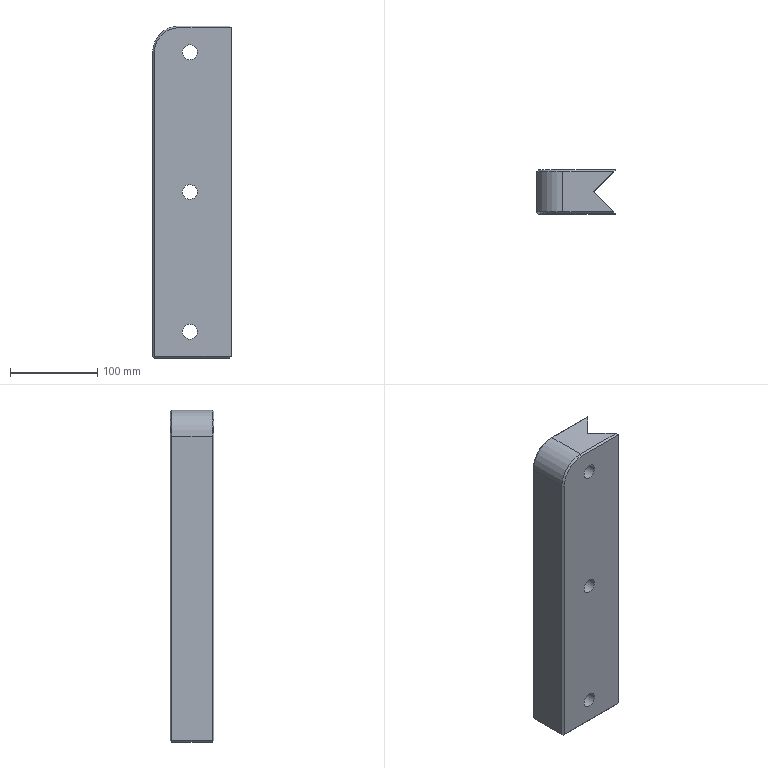Part | Creo | features DATUM PLANE 3, CURVE 2, CHAMFER 1, COORDINATE SYSTEM 1, CUT 1, PROTRUSION 1, ROUND 1 | 1 solid | 23 faces | box 90 x 50 x 380 mm | volume 1426529 mm3 | plane 14 | cylinder 7 | cone 2 | commonest cylinder face diameters 17 x6 60 x1
STEP:
#1=CARTESIAN_POINT('',(0.,0.,0.));
#2=DIRECTION('',(0.,0.,1.));
#3=DIRECTION('',(1.,0.,0.));
#4=AXIS2_PLACEMENT_3D('',#1,#2,#3);
#5=CARTESIAN_POINT('',(-40.5,23.,0.));
#6=VERTEX_POINT('',#5);
#7=CARTESIAN_POINT('',(45.5,23.,0.));
#8=VERTEX_POINT('',#7);
#9=CARTESIAN_POINT('',(-40.5,23.,0.));
#10=DIRECTION('',(1.,0.,0.));
#11=VECTOR('',#10,86.);
#12=LINE('',#9,#11);
#13=EDGE_CURVE('',#6,#8,#12,.T.);
#14=ORIENTED_EDGE('',*,*,#13,.F.);
#15=CARTESIAN_POINT('',(-40.5,-23.,0.));
#16=VERTEX_POINT('',#15);
#17=CARTESIAN_POINT('',(-40.5,-23.,0.));
#18=DIRECTION('',(0.,1.,0.));
#19=VECTOR('',#18,46.);
#20=LINE('',#17,#19);
#21=EDGE_CURVE('',#16,#6,#20,.T.);
#22=ORIENTED_EDGE('',*,*,#21,.F.);
#23=CARTESIAN_POINT('',(45.5,-23.,0.));
#24=VERTEX_POINT('',#23);
#25=CARTESIAN_POINT('',(45.5,-23.,0.));
#26=DIRECTION('',(-1.,0.,0.));
#27=VECTOR('',#26,86.);
#28=LINE('',#25,#27);
#29=EDGE_CURVE('',#24,#16,#28,.T.);
#30=ORIENTED_EDGE('',*,*,#29,.F.);
#31=CARTESIAN_POINT('',(22.5,0.,0.));
#32=VERTEX_POINT('',#31);
#33=CARTESIAN_POINT('',(45.5,-23.,0.));
#34=DIRECTION('',(-0.7071,0.7071,0.));
#35=VECTOR('',#34,32.527);
#36=LINE('',#33,#35);
#37=EDGE_CURVE('',#24,#32,#36,.T.);
#38=ORIENTED_EDGE('',*,*,#37,.T.);
#39=CARTESIAN_POINT('',(22.5,0.,0.));
#40=DIRECTION('',(0.7071,0.7071,0.));
#41=VECTOR('',#40,32.527);
#42=LINE('',#39,#41);
#43=EDGE_CURVE('',#32,#8,#42,.T.);
#44=ORIENTED_EDGE('',*,*,#43,.T.);
#45=EDGE_LOOP('',(#14,#22,#30,#38,#44));
#46=FACE_OUTER_BOUND('',#45,.F.);
#47=CARTESIAN_POINT('',(0.,0.,0.));
#48=DIRECTION('',(0.,0.,1.));
#49=DIRECTION('',(1.,0.,0.));
#50=AXIS2_PLACEMENT_3D('',#47,#48,#49);
#51=PLANE('',#50);
#52=ADVANCED_FACE('',(#46),#51,.F.);
#53=CARTESIAN_POINT('',(47.5,25.,2.));
#54=VERTEX_POINT('',#53);
#55=CARTESIAN_POINT('',(45.5,23.,0.));
#56=DIRECTION('',(0.5774,0.5774,0.5774));
#57=VECTOR('',#56,3.464);
#58=LINE('',#55,#57);
#59=EDGE_CURVE('',#8,#54,#58,.T.);
#60=ORIENTED_EDGE('',*,*,#59,.T.);
#61=CARTESIAN_POINT('',(-40.5,25.,2.));
#62=VERTEX_POINT('',#61);
#63=CARTESIAN_POINT('',(-40.5,25.,2.));
#64=DIRECTION('',(1.,0.,0.));
#65=VECTOR('',#64,88.);
#66=LINE('',#63,#65);
#67=EDGE_CURVE('',#62,#54,#66,.T.);
#68=ORIENTED_EDGE('',*,*,#67,.F.);
#69=CARTESIAN_POINT('',(-41.5,24.,1.));
#70=VERTEX_POINT('',#69);
#71=CARTESIAN_POINT('',(-40.5,25.,2.));
#72=DIRECTION('',(-0.5774,-0.5774,-0.5774));
#73=VECTOR('',#72,1.732);
#74=LINE('',#71,#73);
#75=EDGE_CURVE('',#62,#70,#74,.T.);
#76=ORIENTED_EDGE('',*,*,#75,.T.);
#77=CARTESIAN_POINT('',(-40.5,23.,0.));
#78=DIRECTION('',(-0.5774,0.5774,0.5774));
#79=VECTOR('',#78,1.732);
#80=LINE('',#77,#79);
#81=EDGE_CURVE('',#6,#70,#80,.T.);
#82=ORIENTED_EDGE('',*,*,#81,.F.);
#83=ORIENTED_EDGE('',*,*,#13,.T.);
#84=EDGE_LOOP('',(#60,#68,#76,#82,#83));
#85=FACE_OUTER_BOUND('',#84,.F.);
#86=CARTESIAN_POINT('',(1.5,24.,1.));
#87=DIRECTION('',(0.,0.7071,-0.7071));
#88=DIRECTION('',(0.,0.7071,0.7071));
#89=AXIS2_PLACEMENT_3D('',#86,#87,#88);
#90=PLANE('',#89);
#91=ADVANCED_FACE('',(#85),#90,.T.);
#92=ORIENTED_EDGE('',*,*,#59,.F.);
#93=ORIENTED_EDGE('',*,*,#43,.F.);
#94=CARTESIAN_POINT('',(22.5,0.,380.));
#95=VERTEX_POINT('',#94);
#96=CARTESIAN_POINT('',(22.5,0.,0.));
#97=DIRECTION('',(0.,0.,1.));
#98=VECTOR('',#97,380.);
#99=LINE('',#96,#98);
#100=EDGE_CURVE('',#32,#95,#99,.T.);
#101=ORIENTED_EDGE('',*,*,#100,.T.);
#102=CARTESIAN_POINT('',(45.5,23.,380.));
#103=VERTEX_POINT('',#102);
#104=CARTESIAN_POINT('',(22.5,0.,380.));
#105=DIRECTION('',(0.7071,0.7071,0.));
#106=VECTOR('',#105,32.527);
#107=LINE('',#104,#106);
#108=EDGE_CURVE('',#95,#103,#107,.T.);
#109=ORIENTED_EDGE('',*,*,#108,.T.);
#110=CARTESIAN_POINT('',(47.5,25.,378.));
#111=VERTEX_POINT('',#110);
#112=CARTESIAN_POINT('',(47.5,25.,378.));
#113=DIRECTION('',(-0.5774,-0.5774,0.5774));
#114=VECTOR('',#113,3.464);
#115=LINE('',#112,#114);
#116=EDGE_CURVE('',#111,#103,#115,.T.);
#117=ORIENTED_EDGE('',*,*,#116,.F.);
#118=CARTESIAN_POINT('',(47.5,25.,2.));
#119=DIRECTION('',(0.,0.,1.));
#120=VECTOR('',#119,376.);
#121=LINE('',#118,#120);
#122=EDGE_CURVE('',#54,#111,#121,.T.);
#123=ORIENTED_EDGE('',*,*,#122,.F.);
#124=EDGE_LOOP('',(#92,#93,#101,#109,#117,#123));
#125=FACE_OUTER_BOUND('',#124,.F.);
#126=CARTESIAN_POINT('',(22.5,0.,0.));
#127=DIRECTION('',(0.7071,-0.7071,0.));
#128=DIRECTION('',(0.7071,0.7071,0.));
#129=AXIS2_PLACEMENT_3D('',#126,#127,#128);
#130=PLANE('',#129);
#131=ADVANCED_FACE('',(#125),#130,.T.);
#132=CARTESIAN_POINT('',(47.5,-25.,2.));
#133=VERTEX_POINT('',#132);
#134=CARTESIAN_POINT('',(47.5,-25.,2.));
#135=DIRECTION('',(-0.5774,0.5774,-0.5774));
#136=VECTOR('',#135,3.464);
#137=LINE('',#134,#136);
#138=EDGE_CURVE('',#133,#24,#137,.T.);
#139=ORIENTED_EDGE('',*,*,#138,.F.);
#140=CARTESIAN_POINT('',(47.5,-25.,378.));
#141=VERTEX_POINT('',#140);
#142=CARTESIAN_POINT('',(47.5,-25.,2.));
#143=DIRECTION('',(0.,0.,1.));
#144=VECTOR('',#143,376.);
#145=LINE('',#142,#144);
#146=EDGE_CURVE('',#133,#141,#145,.T.);
#147=ORIENTED_EDGE('',*,*,#146,.T.);
#148=CARTESIAN_POINT('',(45.5,-23.,380.));
#149=VERTEX_POINT('',#148);
#150=CARTESIAN_POINT('',(45.5,-23.,380.));
#151=DIRECTION('',(0.5774,-0.5774,-0.5774));
#152=VECTOR('',#151,3.464);
#153=LINE('',#150,#152);
#154=EDGE_CURVE('',#149,#141,#153,.T.);
#155=ORIENTED_EDGE('',*,*,#154,.F.);
#156=CARTESIAN_POINT('',(45.5,-23.,380.));
#157=DIRECTION('',(-0.7071,0.7071,0.));
#158=VECTOR('',#157,32.527);
#159=LINE('',#156,#158);
#160=EDGE_CURVE('',#149,#95,#159,.T.);
#161=ORIENTED_EDGE('',*,*,#160,.T.);
#162=ORIENTED_EDGE('',*,*,#100,.F.);
#163=ORIENTED_EDGE('',*,*,#37,.F.);
#164=EDGE_LOOP('',(#139,#147,#155,#161,#162,#163));
#165=FACE_OUTER_BOUND('',#164,.F.);
#166=CARTESIAN_POINT('',(47.5,-25.,0.));
#167=DIRECTION('',(0.7071,0.7071,0.));
#168=DIRECTION('',(-0.7071,0.7071,0.));
#169=AXIS2_PLACEMENT_3D('',#166,#167,#168);
#170=PLANE('',#169);
#171=ADVANCED_FACE('',(#165),#170,.T.);
#172=ORIENTED_EDGE('',*,*,#138,.T.);
#173=ORIENTED_EDGE('',*,*,#29,.T.);
#174=CARTESIAN_POINT('',(-41.5,-24.,1.));
#175=VERTEX_POINT('',#174);
#176=CARTESIAN_POINT('',(-41.5,-24.,1.));
#177=DIRECTION('',(0.5774,0.5774,-0.5774));
#178=VECTOR('',#177,1.732);
#179=LINE('',#176,#178);
#180=EDGE_CURVE('',#175,#16,#179,.T.);
#181=ORIENTED_EDGE('',*,*,#180,.F.);
#182=CARTESIAN_POINT('',(-40.5,-25.,2.));
#183=VERTEX_POINT('',#182);
#184=CARTESIAN_POINT('',(-40.5,-25.,2.));
#185=DIRECTION('',(-0.5774,0.5774,-0.5774));
#186=VECTOR('',#185,1.732);
#187=LINE('',#184,#186);
#188=EDGE_CURVE('',#183,#175,#187,.T.);
#189=ORIENTED_EDGE('',*,*,#188,.F.);
#190=CARTESIAN_POINT('',(47.5,-25.,2.));
#191=DIRECTION('',(-1.,0.,0.));
#192=VECTOR('',#191,88.);
#193=LINE('',#190,#192);
#194=EDGE_CURVE('',#133,#183,#193,.T.);
#195=ORIENTED_EDGE('',*,*,#194,.F.);
#196=EDGE_LOOP('',(#172,#173,#181,#189,#195));
#197=FACE_OUTER_BOUND('',#196,.F.);
#198=CARTESIAN_POINT('',(1.5,-24.,1.));
#199=DIRECTION('',(0.,-0.7071,-0.7071));
#200=DIRECTION('',(0.,-0.7071,0.7071));
#201=AXIS2_PLACEMENT_3D('',#198,#199,#200);
#202=PLANE('',#201);
#203=ADVANCED_FACE('',(#197),#202,.T.);
#204=CARTESIAN_POINT('',(-42.5,-23.,2.));
#205=VERTEX_POINT('',#204);
#206=CARTESIAN_POINT('',(-42.5,23.,2.));
#207=VERTEX_POINT('',#206);
#208=CARTESIAN_POINT('',(-42.5,-23.,2.));
#209=DIRECTION('',(0.,1.,0.));
#210=VECTOR('',#209,46.);
#211=LINE('',#208,#210);
#212=EDGE_CURVE('',#205,#207,#211,.T.);
#213=ORIENTED_EDGE('',*,*,#212,.F.);
#214=CARTESIAN_POINT('',(-42.5,-23.,2.));
#215=DIRECTION('',(0.5774,-0.5774,-0.5774));
#216=VECTOR('',#215,1.732);
#217=LINE('',#214,#216);
#218=EDGE_CURVE('',#205,#175,#217,.T.);
#219=ORIENTED_EDGE('',*,*,#218,.T.);
#220=ORIENTED_EDGE('',*,*,#180,.T.);
#221=ORIENTED_EDGE('',*,*,#21,.T.);
#222=ORIENTED_EDGE('',*,*,#81,.T.);
#223=CARTESIAN_POINT('',(-41.5,24.,1.));
#224=DIRECTION('',(-0.5774,-0.5774,0.5774));
#225=VECTOR('',#224,1.732);
#226=LINE('',#223,#225);
#227=EDGE_CURVE('',#70,#207,#226,.T.);
#228=ORIENTED_EDGE('',*,*,#227,.T.);
#229=EDGE_LOOP('',(#213,#219,#220,#221,#222,#228));
#230=FACE_OUTER_BOUND('',#229,.F.);
#231=CARTESIAN_POINT('',(-41.5,0.,1.));
#232=DIRECTION('',(-0.7071,0.,-0.7071));
#233=DIRECTION('',(-0.7071,0.,0.7071));
#234=AXIS2_PLACEMENT_3D('',#231,#232,#233);
#235=PLANE('',#234);
#236=ADVANCED_FACE('',(#230),#235,.T.);
#237=CARTESIAN_POINT('',(-42.5,23.,350.));
#238=VERTEX_POINT('',#237);
#239=CARTESIAN_POINT('',(-42.5,23.,350.));
#240=DIRECTION('',(0.,0.,-1.));
#241=VECTOR('',#240,348.);
#242=LINE('',#239,#241);
#243=EDGE_CURVE('',#238,#207,#242,.T.);
#244=ORIENTED_EDGE('',*,*,#243,.F.);
#245=CARTESIAN_POINT('',(-42.5,-23.,350.));
#246=VERTEX_POINT('',#245);
#247=CARTESIAN_POINT('',(-42.5,23.,350.));
#248=DIRECTION('',(0.,-1.,0.));
#249=VECTOR('',#248,46.);
#250=LINE('',#247,#249);
#251=EDGE_CURVE('',#238,#246,#250,.T.);
#252=ORIENTED_EDGE('',*,*,#251,.T.);
#253=CARTESIAN_POINT('',(-42.5,-23.,350.));
#254=DIRECTION('',(0.,0.,-1.));
#255=VECTOR('',#254,348.);
#256=LINE('',#253,#255);
#257=EDGE_CURVE('',#246,#205,#256,.T.);
#258=ORIENTED_EDGE('',*,*,#257,.T.);
#259=ORIENTED_EDGE('',*,*,#212,.T.);
#260=EDGE_LOOP('',(#244,#252,#258,#259));
#261=FACE_OUTER_BOUND('',#260,.F.);
#262=CARTESIAN_POINT('',(-42.5,25.,0.));
#263=DIRECTION('',(-1.,0.,0.));
#264=DIRECTION('',(0.,-1.,0.));
#265=AXIS2_PLACEMENT_3D('',#262,#263,#264);
#266=PLANE('',#265);
#267=ADVANCED_FACE('',(#261),#266,.T.);
#268=CARTESIAN_POINT('',(-40.5,25.,350.));
#269=VERTEX_POINT('',#268);
#270=CARTESIAN_POINT('',(-40.5,25.,350.));
#271=DIRECTION('',(0.,0.,-1.));
#272=VECTOR('',#271,348.);
#273=LINE('',#270,#272);
#274=EDGE_CURVE('',#269,#62,#273,.T.);
#275=ORIENTED_EDGE('',*,*,#274,.F.);
#276=CARTESIAN_POINT('',(-42.5,23.,350.));
#277=DIRECTION('',(0.7071,0.7071,-0.00000001));
#278=VECTOR('',#277,2.828);
#279=LINE('',#276,#278);
#280=EDGE_CURVE('',#238,#269,#279,.T.);
#281=ORIENTED_EDGE('',*,*,#280,.F.);
#282=ORIENTED_EDGE('',*,*,#243,.T.);
#283=ORIENTED_EDGE('',*,*,#227,.F.);
#284=ORIENTED_EDGE('',*,*,#75,.F.);
#285=EDGE_LOOP('',(#275,#281,#282,#283,#284));
#286=FACE_OUTER_BOUND('',#285,.F.);
#287=CARTESIAN_POINT('',(-41.5,24.,175.));
#288=DIRECTION('',(-0.7071,0.7071,0.));
#289=DIRECTION('',(0.7071,0.7071,0.));
#290=AXIS2_PLACEMENT_3D('',#287,#288,#289);
#291=PLANE('',#290);
#292=ADVANCED_FACE('',(#286),#291,.T.);
#293=ORIENTED_EDGE('',*,*,#67,.T.);
#294=ORIENTED_EDGE('',*,*,#122,.T.);
#295=CARTESIAN_POINT('',(-12.5,25.,378.));
#296=VERTEX_POINT('',#295);
#297=CARTESIAN_POINT('',(47.5,25.,378.));
#298=DIRECTION('',(-1.,0.,0.));
#299=VECTOR('',#298,60.);
#300=LINE('',#297,#299);
#301=EDGE_CURVE('',#111,#296,#300,.T.);
#302=ORIENTED_EDGE('',*,*,#301,.T.);
#303=CARTESIAN_POINT('',(-12.5,25.,350.));
#304=DIRECTION('',(0.,-1.,0.));
#305=DIRECTION('',(0.,0.,1.));
#306=AXIS2_PLACEMENT_3D('',#303,#304,#305);
#307=CIRCLE('',#306,28.);
#308=EDGE_CURVE('',#296,#269,#307,.T.);
#309=ORIENTED_EDGE('',*,*,#308,.T.);
#310=ORIENTED_EDGE('',*,*,#274,.T.);
#311=EDGE_LOOP('',(#293,#294,#302,#309,#310));
#312=FACE_OUTER_BOUND('',#311,.F.);
#313=CARTESIAN_POINT('',(8.5,25.,190.));
#314=VERTEX_POINT('',#313);
#315=CARTESIAN_POINT('',(-8.5,25.,190.));
#316=VERTEX_POINT('',#315);
#317=CARTESIAN_POINT('',(0.,25.,190.));
#318=DIRECTION('',(0.,-1.,0.));
#319=DIRECTION('',(1.,0.,0.));
#320=AXIS2_PLACEMENT_3D('',#317,#318,#319);
#321=CIRCLE('',#320,8.5);
#322=EDGE_CURVE('',#314,#316,#321,.T.);
#323=ORIENTED_EDGE('',*,*,#322,.F.);
#324=CARTESIAN_POINT('',(0.,25.,190.));
#325=DIRECTION('',(0.,-1.,0.));
#326=DIRECTION('',(-1.,0.,0.));
#327=AXIS2_PLACEMENT_3D('',#324,#325,#326);
#328=CIRCLE('',#327,8.5);
#329=EDGE_CURVE('',#316,#314,#328,.T.);
#330=ORIENTED_EDGE('',*,*,#329,.F.);
#331=EDGE_LOOP('',(#323,#330));
#332=FACE_BOUND('',#331,.F.);
#333=CARTESIAN_POINT('',(8.5,25.,30.));
#334=VERTEX_POINT('',#333);
#335=CARTESIAN_POINT('',(-8.5,25.,30.));
#336=VERTEX_POINT('',#335);
#337=CARTESIAN_POINT('',(0.,25.,30.));
#338=DIRECTION('',(0.,-1.,0.));
#339=DIRECTION('',(1.,0.,0.));
#340=AXIS2_PLACEMENT_3D('',#337,#338,#339);
#341=CIRCLE('',#340,8.5);
#342=EDGE_CURVE('',#334,#336,#341,.T.);
#343=ORIENTED_EDGE('',*,*,#342,.F.);
#344=CARTESIAN_POINT('',(0.,25.,30.));
#345=DIRECTION('',(0.,-1.,0.));
#346=DIRECTION('',(-1.,0.,0.));
#347=AXIS2_PLACEMENT_3D('',#344,#345,#346);
#348=CIRCLE('',#347,8.5);
#349=EDGE_CURVE('',#336,#334,#348,.T.);
#350=ORIENTED_EDGE('',*,*,#349,.F.);
#351=EDGE_LOOP('',(#343,#350));
#352=FACE_BOUND('',#351,.F.);
#353=CARTESIAN_POINT('',(8.5,25.,350.));
#354=VERTEX_POINT('',#353);
#355=CARTESIAN_POINT('',(-8.5,25.,350.));
#356=VERTEX_POINT('',#355);
#357=CARTESIAN_POINT('',(0.,25.,350.));
#358=DIRECTION('',(0.,-1.,0.));
#359=DIRECTION('',(1.,0.,0.));
#360=AXIS2_PLACEMENT_3D('',#357,#358,#359);
#361=CIRCLE('',#360,8.5);
#362=EDGE_CURVE('',#354,#356,#361,.T.);
#363=ORIENTED_EDGE('',*,*,#362,.F.);
#364=CARTESIAN_POINT('',(0.,25.,350.));
#365=DIRECTION('',(0.,-1.,0.));
#366=DIRECTION('',(-1.,0.,0.));
#367=AXIS2_PLACEMENT_3D('',#364,#365,#366);
#368=CIRCLE('',#367,8.5);
#369=EDGE_CURVE('',#356,#354,#368,.T.);
#370=ORIENTED_EDGE('',*,*,#369,.F.);
#371=EDGE_LOOP('',(#363,#370));
#372=FACE_BOUND('',#371,.F.);
#373=CARTESIAN_POINT('',(47.5,25.,0.));
#374=DIRECTION('',(0.,1.,0.));
#375=DIRECTION('',(-1.,0.,0.));
#376=AXIS2_PLACEMENT_3D('',#373,#374,#375);
#377=PLANE('',#376);
#378=ADVANCED_FACE('',(#312,#332,#352,#372),#377,.T.);
#379=CARTESIAN_POINT('',(8.5,-25.,350.));
#380=VERTEX_POINT('',#379);
#381=CARTESIAN_POINT('',(-8.5,-25.,350.));
#382=VERTEX_POINT('',#381);
#383=CARTESIAN_POINT('',(0.,-25.,350.));
#384=DIRECTION('',(0.,-1.,0.));
#385=DIRECTION('',(1.,0.,0.));
#386=AXIS2_PLACEMENT_3D('',#383,#384,#385);
#387=CIRCLE('',#386,8.5);
#388=EDGE_CURVE('',#380,#382,#387,.T.);
#389=ORIENTED_EDGE('',*,*,#388,.F.);
#390=CARTESIAN_POINT('',(8.5,-25.,350.));
#391=DIRECTION('',(0.,1.,0.));
#392=VECTOR('',#391,50.);
#393=LINE('',#390,#392);
#394=EDGE_CURVE('',#380,#354,#393,.T.);
#395=ORIENTED_EDGE('',*,*,#394,.T.);
#396=ORIENTED_EDGE('',*,*,#362,.T.);
#397=CARTESIAN_POINT('',(-8.5,-25.,350.));
#398=DIRECTION('',(0.,1.,0.));
#399=VECTOR('',#398,50.);
#400=LINE('',#397,#399);
#401=EDGE_CURVE('',#382,#356,#400,.T.);
#402=ORIENTED_EDGE('',*,*,#401,.F.);
#403=EDGE_LOOP('',(#389,#395,#396,#402));
#404=FACE_OUTER_BOUND('',#403,.F.);
#405=CARTESIAN_POINT('',(0.,-25.,350.));
#406=DIRECTION('',(0.,-1.,0.));
#407=DIRECTION('',(1.,0.,0.));
#408=AXIS2_PLACEMENT_3D('',#405,#406,#407);
#409=CYLINDRICAL_SURFACE('',#408,8.5);
#410=ADVANCED_FACE('',(#404),#409,.F.);
#411=ORIENTED_EDGE('',*,*,#194,.T.);
#412=CARTESIAN_POINT('',(-40.5,-25.,350.));
#413=VERTEX_POINT('',#412);
#414=CARTESIAN_POINT('',(-40.5,-25.,350.));
#415=DIRECTION('',(0.,0.,-1.));
#416=VECTOR('',#415,348.);
#417=LINE('',#414,#416);
#418=EDGE_CURVE('',#413,#183,#417,.T.);
#419=ORIENTED_EDGE('',*,*,#418,.F.);
#420=CARTESIAN_POINT('',(-12.5,-25.,378.));
#421=VERTEX_POINT('',#420);
#422=CARTESIAN_POINT('',(-12.5,-25.,350.));
#423=DIRECTION('',(0.,-1.,0.));
#424=DIRECTION('',(0.,0.,1.));
#425=AXIS2_PLACEMENT_3D('',#422,#423,#424);
#426=CIRCLE('',#425,28.);
#427=EDGE_CURVE('',#421,#413,#426,.T.);
#428=ORIENTED_EDGE('',*,*,#427,.F.);
#429=CARTESIAN_POINT('',(47.5,-25.,378.));
#430=DIRECTION('',(-1.,0.,0.));
#431=VECTOR('',#430,60.);
#432=LINE('',#429,#431);
#433=EDGE_CURVE('',#141,#421,#432,.T.);
#434=ORIENTED_EDGE('',*,*,#433,.F.);
#435=ORIENTED_EDGE('',*,*,#146,.F.);
#436=EDGE_LOOP('',(#411,#419,#428,#434,#435));
#437=FACE_OUTER_BOUND('',#436,.F.);
#438=CARTESIAN_POINT('',(8.5,-25.,190.));
#439=VERTEX_POINT('',#438);
#440=CARTESIAN_POINT('',(-8.5,-25.,190.));
#441=VERTEX_POINT('',#440);
#442=CARTESIAN_POINT('',(0.,-25.,190.));
#443=DIRECTION('',(0.,-1.,0.));
#444=DIRECTION('',(1.,0.,0.));
#445=AXIS2_PLACEMENT_3D('',#442,#443,#444);
#446=CIRCLE('',#445,8.5);
#447=EDGE_CURVE('',#439,#441,#446,.T.);
#448=ORIENTED_EDGE('',*,*,#447,.T.);
#449=CARTESIAN_POINT('',(0.,-25.,190.));
#450=DIRECTION('',(0.,-1.,0.));
#451=DIRECTION('',(-1.,0.,0.));
#452=AXIS2_PLACEMENT_3D('',#449,#450,#451);
#453=CIRCLE('',#452,8.5);
#454=EDGE_CURVE('',#441,#439,#453,.T.);
#455=ORIENTED_EDGE('',*,*,#454,.T.);
#456=EDGE_LOOP('',(#448,#455));
#457=FACE_BOUND('',#456,.F.);
#458=CARTESIAN_POINT('',(8.5,-25.,30.));
#459=VERTEX_POINT('',#458);
#460=CARTESIAN_POINT('',(-8.5,-25.,30.));
#461=VERTEX_POINT('',#460);
#462=CARTESIAN_POINT('',(0.,-25.,30.));
#463=DIRECTION('',(0.,-1.,0.));
#464=DIRECTION('',(1.,0.,0.));
#465=AXIS2_PLACEMENT_3D('',#462,#463,#464);
#466=CIRCLE('',#465,8.5);
#467=EDGE_CURVE('',#459,#461,#466,.T.);
#468=ORIENTED_EDGE('',*,*,#467,.T.);
#469=CARTESIAN_POINT('',(0.,-25.,30.));
#470=DIRECTION('',(0.,-1.,0.));
#471=DIRECTION('',(-1.,0.,0.));
#472=AXIS2_PLACEMENT_3D('',#469,#470,#471);
#473=CIRCLE('',#472,8.5);
#474=EDGE_CURVE('',#461,#459,#473,.T.);
#475=ORIENTED_EDGE('',*,*,#474,.T.);
#476=EDGE_LOOP('',(#468,#475));
#477=FACE_BOUND('',#476,.F.);
#478=ORIENTED_EDGE('',*,*,#388,.T.);
#479=CARTESIAN_POINT('',(0.,-25.,350.));
#480=DIRECTION('',(0.,-1.,0.));
#481=DIRECTION('',(-1.,0.,0.));
#482=AXIS2_PLACEMENT_3D('',#479,#480,#481);
#483=CIRCLE('',#482,8.5);
#484=EDGE_CURVE('',#382,#380,#483,.T.);
#485=ORIENTED_EDGE('',*,*,#484,.T.);
#486=EDGE_LOOP('',(#478,#485));
#487=FACE_BOUND('',#486,.F.);
#488=CARTESIAN_POINT('',(-42.5,-25.,0.));
#489=DIRECTION('',(0.,-1.,0.));
#490=DIRECTION('',(1.,0.,0.));
#491=AXIS2_PLACEMENT_3D('',#488,#489,#490);
#492=PLANE('',#491);
#493=ADVANCED_FACE('',(#437,#457,#477,#487),#492,.T.);
#494=ORIENTED_EDGE('',*,*,#484,.F.);
#495=ORIENTED_EDGE('',*,*,#401,.T.);
#496=ORIENTED_EDGE('',*,*,#369,.T.);
#497=ORIENTED_EDGE('',*,*,#394,.F.);
#498=EDGE_LOOP('',(#494,#495,#496,#497));
#499=FACE_OUTER_BOUND('',#498,.F.);
#500=CARTESIAN_POINT('',(0.,-25.,350.));
#501=DIRECTION('',(0.,-1.,0.));
#502=DIRECTION('',(1.,0.,0.));
#503=AXIS2_PLACEMENT_3D('',#500,#501,#502);
#504=CYLINDRICAL_SURFACE('',#503,8.5);
#505=ADVANCED_FACE('',(#499),#504,.F.);
#506=ORIENTED_EDGE('',*,*,#447,.F.);
#507=CARTESIAN_POINT('',(8.5,-25.,190.));
#508=DIRECTION('',(0.,1.,0.));
#509=VECTOR('',#508,50.);
#510=LINE('',#507,#509);
#511=EDGE_CURVE('',#439,#314,#510,.T.);
#512=ORIENTED_EDGE('',*,*,#511,.T.);
#513=ORIENTED_EDGE('',*,*,#322,.T.);
#514=CARTESIAN_POINT('',(-8.5,-25.,190.));
#515=DIRECTION('',(0.,1.,0.));
#516=VECTOR('',#515,50.);
#517=LINE('',#514,#516);
#518=EDGE_CURVE('',#441,#316,#517,.T.);
#519=ORIENTED_EDGE('',*,*,#518,.F.);
#520=EDGE_LOOP('',(#506,#512,#513,#519));
#521=FACE_OUTER_BOUND('',#520,.F.);
#522=CARTESIAN_POINT('',(0.,-25.,190.));
#523=DIRECTION('',(0.,-1.,0.));
#524=DIRECTION('',(1.,0.,0.));
#525=AXIS2_PLACEMENT_3D('',#522,#523,#524);
#526=CYLINDRICAL_SURFACE('',#525,8.5);
#527=ADVANCED_FACE('',(#521),#526,.F.);
#528=ORIENTED_EDGE('',*,*,#454,.F.);
#529=ORIENTED_EDGE('',*,*,#518,.T.);
#530=ORIENTED_EDGE('',*,*,#329,.T.);
#531=ORIENTED_EDGE('',*,*,#511,.F.);
#532=EDGE_LOOP('',(#528,#529,#530,#531));
#533=FACE_OUTER_BOUND('',#532,.F.);
#534=CARTESIAN_POINT('',(0.,-25.,190.));
#535=DIRECTION('',(0.,-1.,0.));
#536=DIRECTION('',(1.,0.,0.));
#537=AXIS2_PLACEMENT_3D('',#534,#535,#536);
#538=CYLINDRICAL_SURFACE('',#537,8.5);
#539=ADVANCED_FACE('',(#533),#538,.F.);
#540=ORIENTED_EDGE('',*,*,#467,.F.);
#541=CARTESIAN_POINT('',(8.5,-25.,30.));
#542=DIRECTION('',(0.,1.,0.));
#543=VECTOR('',#542,50.);
#544=LINE('',#541,#543);
#545=EDGE_CURVE('',#459,#334,#544,.T.);
#546=ORIENTED_EDGE('',*,*,#545,.T.);
#547=ORIENTED_EDGE('',*,*,#342,.T.);
#548=CARTESIAN_POINT('',(-8.5,-25.,30.));
#549=DIRECTION('',(0.,1.,0.));
#550=VECTOR('',#549,50.);
#551=LINE('',#548,#550);
#552=EDGE_CURVE('',#461,#336,#551,.T.);
#553=ORIENTED_EDGE('',*,*,#552,.F.);
#554=EDGE_LOOP('',(#540,#546,#547,#553));
#555=FACE_OUTER_BOUND('',#554,.F.);
#556=CARTESIAN_POINT('',(0.,-25.,30.));
#557=DIRECTION('',(0.,-1.,0.));
#558=DIRECTION('',(1.,0.,0.));
#559=AXIS2_PLACEMENT_3D('',#556,#557,#558);
#560=CYLINDRICAL_SURFACE('',#559,8.5);
#561=ADVANCED_FACE('',(#555),#560,.F.);
#562=ORIENTED_EDGE('',*,*,#474,.F.);
#563=ORIENTED_EDGE('',*,*,#552,.T.);
#564=ORIENTED_EDGE('',*,*,#349,.T.);
#565=ORIENTED_EDGE('',*,*,#545,.F.);
#566=EDGE_LOOP('',(#562,#563,#564,#565));
#567=FACE_OUTER_BOUND('',#566,.F.);
#568=CARTESIAN_POINT('',(0.,-25.,30.));
#569=DIRECTION('',(0.,-1.,0.));
#570=DIRECTION('',(1.,0.,0.));
#571=AXIS2_PLACEMENT_3D('',#568,#569,#570);
#572=CYLINDRICAL_SURFACE('',#571,8.5);
#573=ADVANCED_FACE('',(#567),#572,.F.);
#574=ORIENTED_EDGE('',*,*,#257,.F.);
#575=CARTESIAN_POINT('',(-40.5,-25.,350.));
#576=DIRECTION('',(-0.7071,0.7071,0.00000001));
#577=VECTOR('',#576,2.828);
#578=LINE('',#575,#577);
#579=EDGE_CURVE('',#413,#246,#578,.T.);
#580=ORIENTED_EDGE('',*,*,#579,.F.);
#581=ORIENTED_EDGE('',*,*,#418,.T.);
#582=ORIENTED_EDGE('',*,*,#188,.T.);
#583=ORIENTED_EDGE('',*,*,#218,.F.);
#584=EDGE_LOOP('',(#574,#580,#581,#582,#583));
#585=FACE_OUTER_BOUND('',#584,.F.);
#586=CARTESIAN_POINT('',(-41.5,-24.,175.));
#587=DIRECTION('',(-0.7071,-0.7071,0.));
#588=DIRECTION('',(-0.7071,0.7071,0.));
#589=AXIS2_PLACEMENT_3D('',#586,#587,#588);
#590=PLANE('',#589);
#591=ADVANCED_FACE('',(#585),#590,.T.);
#592=ORIENTED_EDGE('',*,*,#427,.T.);
#593=ORIENTED_EDGE('',*,*,#579,.T.);
#594=CARTESIAN_POINT('',(-12.5,-23.,380.));
#595=VERTEX_POINT('',#594);
#596=CARTESIAN_POINT('',(-12.5,-23.,350.));
#597=DIRECTION('',(0.,-1.,0.));
#598=DIRECTION('',(0.,0.,1.));
#599=AXIS2_PLACEMENT_3D('',#596,#597,#598);
#600=CIRCLE('',#599,30.);
#601=EDGE_CURVE('',#595,#246,#600,.T.);
#602=ORIENTED_EDGE('',*,*,#601,.F.);
#603=CARTESIAN_POINT('',(-12.5,-25.,378.));
#604=DIRECTION('',(0.000000032,0.7071,0.7071));
#605=VECTOR('',#604,2.828);
#606=LINE('',#603,#605);
#607=EDGE_CURVE('',#421,#595,#606,.T.);
#608=ORIENTED_EDGE('',*,*,#607,.F.);
#609=EDGE_LOOP('',(#592,#593,#602,#608));
#610=FACE_OUTER_BOUND('',#609,.F.);
#611=CARTESIAN_POINT('',(-12.5,-24.,350.));
#612=DIRECTION('',(0.,1.,0.));
#613=DIRECTION('',(0.,0.,-1.));
#614=AXIS2_PLACEMENT_3D('',#611,#612,#613);
#615=CONICAL_SURFACE('',#614,29.,45.);
#616=ADVANCED_FACE('',(#610),#615,.T.);
#617=CARTESIAN_POINT('',(-12.5,23.,380.));
#618=VERTEX_POINT('',#617);
#619=CARTESIAN_POINT('',(-12.5,23.,350.));
#620=DIRECTION('',(0.,-1.,0.));
#621=DIRECTION('',(0.,0.,1.));
#622=AXIS2_PLACEMENT_3D('',#619,#620,#621);
#623=CIRCLE('',#622,30.);
#624=EDGE_CURVE('',#618,#238,#623,.T.);
#625=ORIENTED_EDGE('',*,*,#624,.F.);
#626=CARTESIAN_POINT('',(-12.5,23.,380.));
#627=DIRECTION('',(0.000000003,-1.,0.));
#628=VECTOR('',#627,46.);
#629=LINE('',#626,#628);
#630=EDGE_CURVE('',#618,#595,#629,.T.);
#631=ORIENTED_EDGE('',*,*,#630,.T.);
#632=ORIENTED_EDGE('',*,*,#601,.T.);
#633=ORIENTED_EDGE('',*,*,#251,.F.);
#634=EDGE_LOOP('',(#625,#631,#632,#633));
#635=FACE_OUTER_BOUND('',#634,.F.);
#636=CARTESIAN_POINT('',(-12.5,90.18,350.));
#637=DIRECTION('',(0.,-1.,0.));
#638=DIRECTION('',(0.,0.,1.));
#639=AXIS2_PLACEMENT_3D('',#636,#637,#638);
#640=CYLINDRICAL_SURFACE('',#639,30.);
#641=ADVANCED_FACE('',(#635),#640,.T.);
#642=ORIENTED_EDGE('',*,*,#624,.T.);
#643=ORIENTED_EDGE('',*,*,#280,.T.);
#644=ORIENTED_EDGE('',*,*,#308,.F.);
#645=CARTESIAN_POINT('',(-12.5,23.,380.));
#646=DIRECTION('',(0.000000061,0.7071,-0.7071));
#647=VECTOR('',#646,2.828);
#648=LINE('',#645,#647);
#649=EDGE_CURVE('',#618,#296,#648,.T.);
#650=ORIENTED_EDGE('',*,*,#649,.F.);
#651=EDGE_LOOP('',(#642,#643,#644,#650));
#652=FACE_OUTER_BOUND('',#651,.F.);
#653=CARTESIAN_POINT('',(-12.5,24.,350.));
#654=DIRECTION('',(0.,-1.,0.));
#655=DIRECTION('',(0.,0.,-1.));
#656=AXIS2_PLACEMENT_3D('',#653,#654,#655);
#657=CONICAL_SURFACE('',#656,29.,45.);
#658=ADVANCED_FACE('',(#652),#657,.T.);
#659=ORIENTED_EDGE('',*,*,#116,.T.);
#660=CARTESIAN_POINT('',(45.5,23.,380.));
#661=DIRECTION('',(-1.,0.,0.));
#662=VECTOR('',#661,58.);
#663=LINE('',#660,#662);
#664=EDGE_CURVE('',#103,#618,#663,.T.);
#665=ORIENTED_EDGE('',*,*,#664,.T.);
#666=ORIENTED_EDGE('',*,*,#649,.T.);
#667=ORIENTED_EDGE('',*,*,#301,.F.);
#668=EDGE_LOOP('',(#659,#665,#666,#667));
#669=FACE_OUTER_BOUND('',#668,.F.);
#670=CARTESIAN_POINT('',(16.5,24.,379.));
#671=DIRECTION('',(0.,0.7071,0.7071));
#672=DIRECTION('',(0.,0.7071,-0.7071));
#673=AXIS2_PLACEMENT_3D('',#670,#671,#672);
#674=PLANE('',#673);
#675=ADVANCED_FACE('',(#669),#674,.T.);
#676=ORIENTED_EDGE('',*,*,#664,.F.);
#677=ORIENTED_EDGE('',*,*,#108,.F.);
#678=ORIENTED_EDGE('',*,*,#160,.F.);
#679=CARTESIAN_POINT('',(45.5,-23.,380.));
#680=DIRECTION('',(-1.,0.,0.));
#681=VECTOR('',#680,58.);
#682=LINE('',#679,#681);
#683=EDGE_CURVE('',#149,#595,#682,.T.);
#684=ORIENTED_EDGE('',*,*,#683,.T.);
#685=ORIENTED_EDGE('',*,*,#630,.F.);
#686=EDGE_LOOP('',(#676,#677,#678,#684,#685));
#687=FACE_OUTER_BOUND('',#686,.F.);
#688=CARTESIAN_POINT('',(0.,0.,380.));
#689=DIRECTION('',(0.,0.,1.));
#690=DIRECTION('',(1.,0.,0.));
#691=AXIS2_PLACEMENT_3D('',#688,#689,#690);
#692=PLANE('',#691);
#693=ADVANCED_FACE('',(#687),#692,.T.);
#694=ORIENTED_EDGE('',*,*,#154,.T.);
#695=ORIENTED_EDGE('',*,*,#433,.T.);
#696=ORIENTED_EDGE('',*,*,#607,.T.);
#697=ORIENTED_EDGE('',*,*,#683,.F.);
#698=EDGE_LOOP('',(#694,#695,#696,#697));
#699=FACE_OUTER_BOUND('',#698,.F.);
#700=CARTESIAN_POINT('',(16.5,-24.,379.));
#701=DIRECTION('',(0.,-0.7071,0.7071));
#702=DIRECTION('',(0.,0.7071,0.7071));
#703=AXIS2_PLACEMENT_3D('',#700,#701,#702);
#704=PLANE('',#703);
#705=ADVANCED_FACE('',(#699),#704,.T.);
#706=CLOSED_SHELL('',(#52,#91,#131,#171,#203,#236,#267,#292,#378,#410,#493,#505,#527,#539,#561,#573,#591,#616,#641,#658,#675,#693,#705));
#707=MANIFOLD_SOLID_BREP('',#706);
#708=(LENGTH_UNIT()NAMED_UNIT(*)SI_UNIT(.MILLI.,.METRE.));
#709=UNCERTAINTY_MEASURE_WITH_UNIT(LENGTH_MEASURE(0.03937),#708,'','');
#710=(NAMED_UNIT(*)PLANE_ANGLE_UNIT()SI_UNIT($,.RADIAN.));
#711=PLANE_ANGLE_MEASURE_WITH_UNIT(PLANE_ANGLE_MEASURE(0.01745),#710);
#712=(CONVERSION_BASED_UNIT('DEGREE',#711)NAMED_UNIT(*)PLANE_ANGLE_UNIT());
#713=(NAMED_UNIT(*)SI_UNIT($,.STERADIAN.)SOLID_ANGLE_UNIT());
#714=(GEOMETRIC_REPRESENTATION_CONTEXT(3)GLOBAL_UNCERTAINTY_ASSIGNED_CONTEXT((#709))GLOBAL_UNIT_ASSIGNED_CONTEXT((#708,#712,#713))REPRESENTATION_CONTEXT('',''));
#715=ADVANCED_BREP_SHAPE_REPRESENTATION('',(#4,#707),#714);